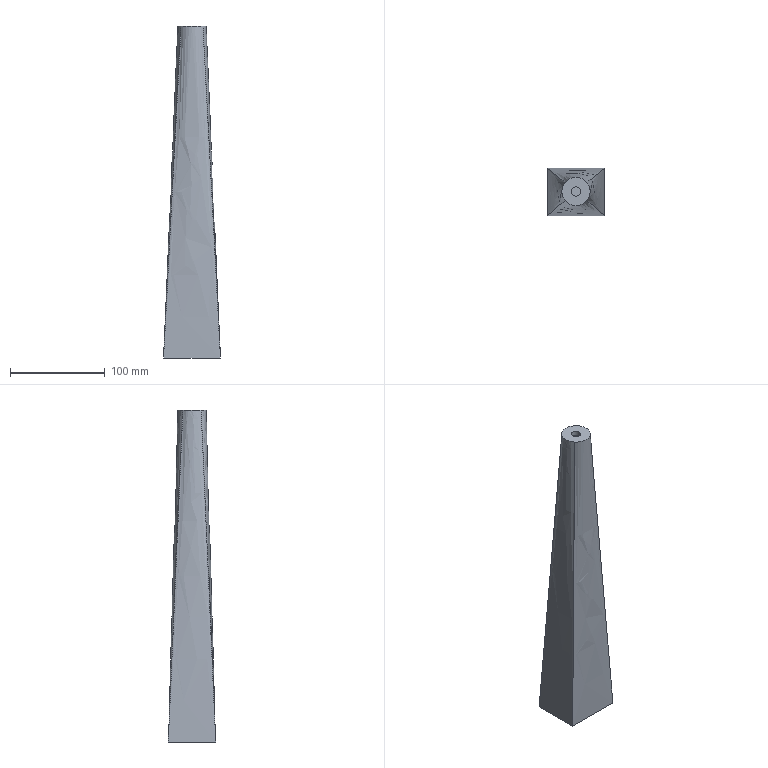Part | SolidWorks | features Blend 1, Cut 1 | 1 solid | 9 faces | box 60 x 50 x 350 mm | volume 603883 mm3 | spline 4 | plane 3 | cylinder 2 | commonest cylinder face diameters 9.779 x2
STEP:
#1=CARTESIAN_POINT('',(-4.89,0.,-5.));
#2=VERTEX_POINT('',#1);
#3=CARTESIAN_POINT('',(4.89,0.,-5.));
#4=VERTEX_POINT('',#3);
#5=CARTESIAN_POINT('',(0.,0.,-5.));
#6=DIRECTION('',(0.,0.,1.));
#7=DIRECTION('',(1.,0.,0.));
#8=AXIS2_PLACEMENT_3D('',#5,#6,#7);
#9=CIRCLE('',#8,4.89);
#10=EDGE_CURVE('',#2,#4,#9,.T.);
#11=ORIENTED_EDGE('',*,*,#10,.F.);
#12=CARTESIAN_POINT('',(-4.89,0.,0.));
#13=VERTEX_POINT('',#12);
#14=CARTESIAN_POINT('',(-4.89,0.,-5.));
#15=DIRECTION('',(0.,0.,1.));
#16=VECTOR('',#15,1000.);
#17=LINE('',#14,#16);
#18=EDGE_CURVE('',#2,#13,#17,.T.);
#19=ORIENTED_EDGE('',*,*,#18,.T.);
#20=CARTESIAN_POINT('',(4.89,0.,0.));
#21=VERTEX_POINT('',#20);
#22=CARTESIAN_POINT('',(0.,0.,0.));
#23=DIRECTION('',(0.,0.,1.));
#24=DIRECTION('',(1.,0.,0.));
#25=AXIS2_PLACEMENT_3D('',#22,#23,#24);
#26=CIRCLE('',#25,4.89);
#27=EDGE_CURVE('',#13,#21,#26,.T.);
#28=ORIENTED_EDGE('',*,*,#27,.T.);
#29=CARTESIAN_POINT('',(4.89,0.,-5.));
#30=DIRECTION('',(0.,0.,1.));
#31=VECTOR('',#30,1000.);
#32=LINE('',#29,#31);
#33=EDGE_CURVE('',#4,#21,#32,.T.);
#34=ORIENTED_EDGE('',*,*,#33,.F.);
#35=EDGE_LOOP('',(#11,#19,#28,#34));
#36=FACE_OUTER_BOUND('',#35,.T.);
#37=CARTESIAN_POINT('',(0.,0.,-5.));
#38=DIRECTION('',(0.,0.,1.));
#39=DIRECTION('',(1.,0.,0.));
#40=AXIS2_PLACEMENT_3D('',#37,#38,#39);
#41=CYLINDRICAL_SURFACE('',#40,4.89);
#42=ADVANCED_FACE('',(#36),#41,.F.);
#43=CARTESIAN_POINT('',(0.,0.,0.));
#44=DIRECTION('',(0.,0.,1.));
#45=DIRECTION('',(1.,0.,0.));
#46=AXIS2_PLACEMENT_3D('',#43,#44,#45);
#47=CIRCLE('',#46,4.89);
#48=EDGE_CURVE('',#21,#13,#47,.T.);
#49=ORIENTED_EDGE('',*,*,#48,.F.);
#50=ORIENTED_EDGE('',*,*,#27,.F.);
#51=EDGE_LOOP('',(#49,#50));
#52=FACE_BOUND('',#51,.T.);
#53=CARTESIAN_POINT('',(11.523,-9.603,0.));
#54=VERTEX_POINT('',#53);
#55=CARTESIAN_POINT('',(11.523,9.603,0.));
#56=VERTEX_POINT('',#55);
#57=CARTESIAN_POINT('',(0.,0.,0.));
#58=DIRECTION('',(0.,0.,1.));
#59=DIRECTION('',(1.,0.,0.));
#60=AXIS2_PLACEMENT_3D('',#57,#58,#59);
#61=CIRCLE('',#60,15.);
#62=EDGE_CURVE('',#54,#56,#61,.T.);
#63=ORIENTED_EDGE('',*,*,#62,.T.);
#64=CARTESIAN_POINT('',(-11.523,9.603,0.));
#65=VERTEX_POINT('',#64);
#66=CARTESIAN_POINT('',(0.,0.,0.));
#67=DIRECTION('',(0.,0.,1.));
#68=DIRECTION('',(1.,0.,0.));
#69=AXIS2_PLACEMENT_3D('',#66,#67,#68);
#70=CIRCLE('',#69,15.);
#71=EDGE_CURVE('',#56,#65,#70,.T.);
#72=ORIENTED_EDGE('',*,*,#71,.T.);
#73=CARTESIAN_POINT('',(-11.523,-9.603,0.));
#74=VERTEX_POINT('',#73);
#75=CARTESIAN_POINT('',(0.,0.,0.));
#76=DIRECTION('',(0.,0.,1.));
#77=DIRECTION('',(1.,0.,0.));
#78=AXIS2_PLACEMENT_3D('',#75,#76,#77);
#79=CIRCLE('',#78,15.);
#80=EDGE_CURVE('',#65,#74,#79,.T.);
#81=ORIENTED_EDGE('',*,*,#80,.T.);
#82=CARTESIAN_POINT('',(0.,0.,0.));
#83=DIRECTION('',(0.,0.,1.));
#84=DIRECTION('',(1.,0.,0.));
#85=AXIS2_PLACEMENT_3D('',#82,#83,#84);
#86=CIRCLE('',#85,15.);
#87=EDGE_CURVE('',#74,#54,#86,.T.);
#88=ORIENTED_EDGE('',*,*,#87,.T.);
#89=EDGE_LOOP('',(#63,#72,#81,#88));
#90=FACE_OUTER_BOUND('',#89,.T.);
#91=CARTESIAN_POINT('',(0.,0.,0.));
#92=DIRECTION('',(0.,0.,1.));
#93=DIRECTION('',(1.,0.,0.));
#94=AXIS2_PLACEMENT_3D('',#91,#92,#93);
#95=PLANE('',#94);
#96=ADVANCED_FACE('',(#52,#90),#95,.T.);
#97=CARTESIAN_POINT('',(30.,-25.,-350.));
#98=VERTEX_POINT('',#97);
#99=CARTESIAN_POINT('',(30.,25.,-350.));
#100=VERTEX_POINT('',#99);
#101=CARTESIAN_POINT('',(30.,25.,-350.));
#102=DIRECTION('',(0.,1.,0.));
#103=VECTOR('',#102,1000.);
#104=LINE('',#101,#103);
#105=EDGE_CURVE('',#98,#100,#104,.T.);
#106=ORIENTED_EDGE('',*,*,#105,.F.);
#107=CARTESIAN_POINT('',(-30.,-25.,-350.));
#108=VERTEX_POINT('',#107);
#109=CARTESIAN_POINT('',(-30.,-25.,-350.));
#110=DIRECTION('',(1.,0.,0.));
#111=VECTOR('',#110,1000.);
#112=LINE('',#109,#111);
#113=EDGE_CURVE('',#108,#98,#112,.T.);
#114=ORIENTED_EDGE('',*,*,#113,.F.);
#115=CARTESIAN_POINT('',(-30.,25.,-350.));
#116=VERTEX_POINT('',#115);
#117=CARTESIAN_POINT('',(-30.,25.,-350.));
#118=DIRECTION('',(0.,-1.,0.));
#119=VECTOR('',#118,1000.);
#120=LINE('',#117,#119);
#121=EDGE_CURVE('',#116,#108,#120,.T.);
#122=ORIENTED_EDGE('',*,*,#121,.F.);
#123=CARTESIAN_POINT('',(-30.,25.,-350.));
#124=DIRECTION('',(-1.,0.,0.));
#125=VECTOR('',#124,1000.);
#126=LINE('',#123,#125);
#127=EDGE_CURVE('',#100,#116,#126,.T.);
#128=ORIENTED_EDGE('',*,*,#127,.F.);
#129=EDGE_LOOP('',(#106,#114,#122,#128));
#130=FACE_OUTER_BOUND('',#129,.T.);
#131=CARTESIAN_POINT('',(0.,0.,-350.));
#132=DIRECTION('',(0.,0.,1.));
#133=DIRECTION('',(1.,0.,0.));
#134=AXIS2_PLACEMENT_3D('',#131,#132,#133);
#135=PLANE('',#134);
#136=ADVANCED_FACE('',(#130),#135,.F.);
#137=ORIENTED_EDGE('',*,*,#127,.T.);
#138=CARTESIAN_POINT('',(-20.762,17.301,-175.));
#139=DIRECTION('',(0.05267,-0.04389,0.9976));
#140=VECTOR('',#139,1000.);
#141=LINE('',#138,#140);
#142=EDGE_CURVE('',#116,#65,#141,.T.);
#143=ORIENTED_EDGE('',*,*,#142,.T.);
#144=ORIENTED_EDGE('',*,*,#71,.F.);
#145=CARTESIAN_POINT('',(20.762,17.301,-175.));
#146=DIRECTION('',(0.05267,0.04389,-0.9976));
#147=VECTOR('',#146,1000.);
#148=LINE('',#145,#147);
#149=EDGE_CURVE('',#56,#100,#148,.T.);
#150=ORIENTED_EDGE('',*,*,#149,.T.);
#151=EDGE_LOOP('',(#137,#143,#144,#150));
#152=FACE_OUTER_BOUND('',#151,.T.);
#153=CARTESIAN_POINT('',(30.,25.,-350.));
#154=CARTESIAN_POINT('',(11.523,9.603,0.));
#155=CARTESIAN_POINT('',(27.5,25.,-350.));
#156=CARTESIAN_POINT('',(10.909,10.34,0.));
#157=CARTESIAN_POINT('',(25.,25.,-350.));
#158=CARTESIAN_POINT('',(10.194,11.053,0.));
#159=CARTESIAN_POINT('',(20.,25.,-350.));
#160=CARTESIAN_POINT('',(8.568,12.357,0.));
#161=CARTESIAN_POINT('',(17.5,25.,-350.));
#162=CARTESIAN_POINT('',(7.655,12.947,0.));
#163=CARTESIAN_POINT('',(12.5,25.,-350.));
#164=CARTESIAN_POINT('',(5.666,13.933,0.));
#165=CARTESIAN_POINT('',(10.,25.,-350.));
#166=CARTESIAN_POINT('',(4.589,14.327,0.));
#167=CARTESIAN_POINT('',(5.,25.,-350.));
#168=CARTESIAN_POINT('',(2.341,14.861,0.));
#169=CARTESIAN_POINT('',(2.5,25.,-350.));
#170=CARTESIAN_POINT('',(1.171,15.,0.));
#171=CARTESIAN_POINT('',(-2.5,25.,-350.));
#172=CARTESIAN_POINT('',(-1.171,15.,0.));
#173=CARTESIAN_POINT('',(-5.,25.,-350.));
#174=CARTESIAN_POINT('',(-2.341,14.861,0.));
#175=CARTESIAN_POINT('',(-10.,25.,-350.));
#176=CARTESIAN_POINT('',(-4.589,14.327,0.));
#177=CARTESIAN_POINT('',(-12.5,25.,-350.));
#178=CARTESIAN_POINT('',(-5.666,13.933,0.));
#179=CARTESIAN_POINT('',(-17.5,25.,-350.));
#180=CARTESIAN_POINT('',(-7.655,12.947,0.));
#181=CARTESIAN_POINT('',(-20.,25.,-350.));
#182=CARTESIAN_POINT('',(-8.568,12.357,0.));
#183=CARTESIAN_POINT('',(-25.,25.,-350.));
#184=CARTESIAN_POINT('',(-10.194,11.053,0.));
#185=CARTESIAN_POINT('',(-27.5,25.,-350.));
#186=CARTESIAN_POINT('',(-10.909,10.34,0.));
#187=CARTESIAN_POINT('',(-30.,25.,-350.));
#188=CARTESIAN_POINT('',(-11.523,9.603,0.));
#189=B_SPLINE_SURFACE_WITH_KNOTS('',3,1,((#153,#154),(#155,#156),(#157,#158),(#159,#160),(#161,#162),(#163,#164),(#165,#166),(#167,#168),(#169,#170),(#171,#172),(#173,#174),(#175,#176),(#177,#178),(#179,#180),(#181,#182),(#183,#184),(#185,#186),(#187,#188)),.UNSPECIFIED.,.F.,.F.,.F.,(4,2,2,2,2,2,2,2,4),(2,2),(0.,0.125,0.25,0.375,0.5,0.625,0.75,0.875,1.),(0.,1.),.UNSPECIFIED.);
#190=ADVANCED_FACE('',(#152),#189,.T.);
#191=ORIENTED_EDGE('',*,*,#121,.T.);
#192=CARTESIAN_POINT('',(-20.762,-17.301,-175.));
#193=DIRECTION('',(0.05267,0.04389,0.9976));
#194=VECTOR('',#193,1000.);
#195=LINE('',#192,#194);
#196=EDGE_CURVE('',#108,#74,#195,.T.);
#197=ORIENTED_EDGE('',*,*,#196,.T.);
#198=ORIENTED_EDGE('',*,*,#80,.F.);
#199=ORIENTED_EDGE('',*,*,#142,.F.);
#200=EDGE_LOOP('',(#191,#197,#198,#199));
#201=FACE_OUTER_BOUND('',#200,.T.);
#202=CARTESIAN_POINT('',(-30.,25.,-350.));
#203=CARTESIAN_POINT('',(-11.523,9.603,0.));
#204=CARTESIAN_POINT('',(-30.,22.917,-350.));
#205=CARTESIAN_POINT('',(-12.036,8.988,0.));
#206=CARTESIAN_POINT('',(-30.,20.833,-350.));
#207=CARTESIAN_POINT('',(-12.514,8.314,0.));
#208=CARTESIAN_POINT('',(-30.,16.667,-350.));
#209=CARTESIAN_POINT('',(-13.366,6.86,0.));
#210=CARTESIAN_POINT('',(-30.,14.583,-350.));
#211=CARTESIAN_POINT('',(-13.741,6.079,0.));
#212=CARTESIAN_POINT('',(-30.,10.417,-350.));
#213=CARTESIAN_POINT('',(-14.355,4.438,0.));
#214=CARTESIAN_POINT('',(-30.,8.333,-350.));
#215=CARTESIAN_POINT('',(-14.595,3.576,0.));
#216=CARTESIAN_POINT('',(-30.,4.167,-350.));
#217=CARTESIAN_POINT('',(-14.917,1.81,0.));
#218=CARTESIAN_POINT('',(-30.,2.083,-350.));
#219=CARTESIAN_POINT('',(-15.,0.9051,0.));
#220=CARTESIAN_POINT('',(-30.,-2.083,-350.));
#221=CARTESIAN_POINT('',(-15.,-0.9051,0.));
#222=CARTESIAN_POINT('',(-30.,-4.167,-350.));
#223=CARTESIAN_POINT('',(-14.917,-1.81,0.));
#224=CARTESIAN_POINT('',(-30.,-8.333,-350.));
#225=CARTESIAN_POINT('',(-14.595,-3.576,0.));
#226=CARTESIAN_POINT('',(-30.,-10.417,-350.));
#227=CARTESIAN_POINT('',(-14.355,-4.438,0.));
#228=CARTESIAN_POINT('',(-30.,-14.583,-350.));
#229=CARTESIAN_POINT('',(-13.741,-6.079,0.));
#230=CARTESIAN_POINT('',(-30.,-16.667,-350.));
#231=CARTESIAN_POINT('',(-13.366,-6.86,0.));
#232=CARTESIAN_POINT('',(-30.,-20.833,-350.));
#233=CARTESIAN_POINT('',(-12.514,-8.314,0.));
#234=CARTESIAN_POINT('',(-30.,-22.917,-350.));
#235=CARTESIAN_POINT('',(-12.036,-8.988,0.));
#236=CARTESIAN_POINT('',(-30.,-25.,-350.));
#237=CARTESIAN_POINT('',(-11.523,-9.603,0.));
#238=B_SPLINE_SURFACE_WITH_KNOTS('',3,1,((#202,#203),(#204,#205),(#206,#207),(#208,#209),(#210,#211),(#212,#213),(#214,#215),(#216,#217),(#218,#219),(#220,#221),(#222,#223),(#224,#225),(#226,#227),(#228,#229),(#230,#231),(#232,#233),(#234,#235),(#236,#237)),.UNSPECIFIED.,.F.,.F.,.F.,(4,2,2,2,2,2,2,2,4),(2,2),(0.,0.125,0.25,0.375,0.5,0.625,0.75,0.875,1.),(0.,1.),.UNSPECIFIED.);
#239=ADVANCED_FACE('',(#201),#238,.T.);
#240=ORIENTED_EDGE('',*,*,#105,.T.);
#241=ORIENTED_EDGE('',*,*,#149,.F.);
#242=ORIENTED_EDGE('',*,*,#62,.F.);
#243=CARTESIAN_POINT('',(20.762,-17.301,-175.));
#244=DIRECTION('',(-0.05267,0.04389,0.9976));
#245=VECTOR('',#244,1000.);
#246=LINE('',#243,#245);
#247=EDGE_CURVE('',#98,#54,#246,.T.);
#248=ORIENTED_EDGE('',*,*,#247,.F.);
#249=EDGE_LOOP('',(#240,#241,#242,#248));
#250=FACE_OUTER_BOUND('',#249,.T.);
#251=CARTESIAN_POINT('',(30.,-25.,-350.));
#252=CARTESIAN_POINT('',(11.523,-9.603,0.));
#253=CARTESIAN_POINT('',(30.,-22.917,-350.));
#254=CARTESIAN_POINT('',(12.036,-8.988,0.));
#255=CARTESIAN_POINT('',(30.,-20.833,-350.));
#256=CARTESIAN_POINT('',(12.514,-8.314,0.));
#257=CARTESIAN_POINT('',(30.,-16.667,-350.));
#258=CARTESIAN_POINT('',(13.366,-6.86,0.));
#259=CARTESIAN_POINT('',(30.,-14.583,-350.));
#260=CARTESIAN_POINT('',(13.741,-6.079,0.));
#261=CARTESIAN_POINT('',(30.,-10.417,-350.));
#262=CARTESIAN_POINT('',(14.355,-4.438,0.));
#263=CARTESIAN_POINT('',(30.,-8.333,-350.));
#264=CARTESIAN_POINT('',(14.595,-3.576,0.));
#265=CARTESIAN_POINT('',(30.,-4.167,-350.));
#266=CARTESIAN_POINT('',(14.917,-1.81,0.));
#267=CARTESIAN_POINT('',(30.,-2.083,-350.));
#268=CARTESIAN_POINT('',(15.,-0.9051,0.));
#269=CARTESIAN_POINT('',(30.,2.083,-350.));
#270=CARTESIAN_POINT('',(15.,0.9051,0.));
#271=CARTESIAN_POINT('',(30.,4.167,-350.));
#272=CARTESIAN_POINT('',(14.917,1.81,0.));
#273=CARTESIAN_POINT('',(30.,8.333,-350.));
#274=CARTESIAN_POINT('',(14.595,3.576,0.));
#275=CARTESIAN_POINT('',(30.,10.417,-350.));
#276=CARTESIAN_POINT('',(14.355,4.438,0.));
#277=CARTESIAN_POINT('',(30.,14.583,-350.));
#278=CARTESIAN_POINT('',(13.741,6.079,0.));
#279=CARTESIAN_POINT('',(30.,16.667,-350.));
#280=CARTESIAN_POINT('',(13.366,6.86,0.));
#281=CARTESIAN_POINT('',(30.,20.833,-350.));
#282=CARTESIAN_POINT('',(12.514,8.314,0.));
#283=CARTESIAN_POINT('',(30.,22.917,-350.));
#284=CARTESIAN_POINT('',(12.036,8.988,0.));
#285=CARTESIAN_POINT('',(30.,25.,-350.));
#286=CARTESIAN_POINT('',(11.523,9.603,0.));
#287=B_SPLINE_SURFACE_WITH_KNOTS('',3,1,((#251,#252),(#253,#254),(#255,#256),(#257,#258),(#259,#260),(#261,#262),(#263,#264),(#265,#266),(#267,#268),(#269,#270),(#271,#272),(#273,#274),(#275,#276),(#277,#278),(#279,#280),(#281,#282),(#283,#284),(#285,#286)),.UNSPECIFIED.,.F.,.F.,.F.,(4,2,2,2,2,2,2,2,4),(2,2),(0.,0.125,0.25,0.375,0.5,0.625,0.75,0.875,1.),(0.,1.),.UNSPECIFIED.);
#288=ADVANCED_FACE('',(#250),#287,.T.);
#289=ORIENTED_EDGE('',*,*,#113,.T.);
#290=ORIENTED_EDGE('',*,*,#247,.T.);
#291=ORIENTED_EDGE('',*,*,#87,.F.);
#292=ORIENTED_EDGE('',*,*,#196,.F.);
#293=EDGE_LOOP('',(#289,#290,#291,#292));
#294=FACE_OUTER_BOUND('',#293,.T.);
#295=CARTESIAN_POINT('',(-30.,-25.,-350.));
#296=CARTESIAN_POINT('',(-11.523,-9.603,0.));
#297=CARTESIAN_POINT('',(-27.5,-25.,-350.));
#298=CARTESIAN_POINT('',(-10.909,-10.34,0.));
#299=CARTESIAN_POINT('',(-25.,-25.,-350.));
#300=CARTESIAN_POINT('',(-10.194,-11.053,0.));
#301=CARTESIAN_POINT('',(-20.,-25.,-350.));
#302=CARTESIAN_POINT('',(-8.568,-12.357,0.));
#303=CARTESIAN_POINT('',(-17.5,-25.,-350.));
#304=CARTESIAN_POINT('',(-7.655,-12.947,0.));
#305=CARTESIAN_POINT('',(-12.5,-25.,-350.));
#306=CARTESIAN_POINT('',(-5.666,-13.933,0.));
#307=CARTESIAN_POINT('',(-10.,-25.,-350.));
#308=CARTESIAN_POINT('',(-4.589,-14.327,0.));
#309=CARTESIAN_POINT('',(-5.,-25.,-350.));
#310=CARTESIAN_POINT('',(-2.341,-14.861,0.));
#311=CARTESIAN_POINT('',(-2.5,-25.,-350.));
#312=CARTESIAN_POINT('',(-1.171,-15.,0.));
#313=CARTESIAN_POINT('',(2.5,-25.,-350.));
#314=CARTESIAN_POINT('',(1.171,-15.,0.));
#315=CARTESIAN_POINT('',(5.,-25.,-350.));
#316=CARTESIAN_POINT('',(2.341,-14.861,0.));
#317=CARTESIAN_POINT('',(10.,-25.,-350.));
#318=CARTESIAN_POINT('',(4.589,-14.327,0.));
#319=CARTESIAN_POINT('',(12.5,-25.,-350.));
#320=CARTESIAN_POINT('',(5.666,-13.933,0.));
#321=CARTESIAN_POINT('',(17.5,-25.,-350.));
#322=CARTESIAN_POINT('',(7.655,-12.947,0.));
#323=CARTESIAN_POINT('',(20.,-25.,-350.));
#324=CARTESIAN_POINT('',(8.568,-12.357,0.));
#325=CARTESIAN_POINT('',(25.,-25.,-350.));
#326=CARTESIAN_POINT('',(10.194,-11.053,0.));
#327=CARTESIAN_POINT('',(27.5,-25.,-350.));
#328=CARTESIAN_POINT('',(10.909,-10.34,0.));
#329=CARTESIAN_POINT('',(30.,-25.,-350.));
#330=CARTESIAN_POINT('',(11.523,-9.603,0.));
#331=B_SPLINE_SURFACE_WITH_KNOTS('',3,1,((#295,#296),(#297,#298),(#299,#300),(#301,#302),(#303,#304),(#305,#306),(#307,#308),(#309,#310),(#311,#312),(#313,#314),(#315,#316),(#317,#318),(#319,#320),(#321,#322),(#323,#324),(#325,#326),(#327,#328),(#329,#330)),.UNSPECIFIED.,.F.,.F.,.F.,(4,2,2,2,2,2,2,2,4),(2,2),(0.,0.125,0.25,0.375,0.5,0.625,0.75,0.875,1.),(0.,1.),.UNSPECIFIED.);
#332=ADVANCED_FACE('',(#294),#331,.T.);
#333=ORIENTED_EDGE('',*,*,#18,.F.);
#334=CARTESIAN_POINT('',(0.,0.,-5.));
#335=DIRECTION('',(0.,0.,1.));
#336=DIRECTION('',(1.,0.,0.));
#337=AXIS2_PLACEMENT_3D('',#334,#335,#336);
#338=CIRCLE('',#337,4.89);
#339=EDGE_CURVE('',#4,#2,#338,.T.);
#340=ORIENTED_EDGE('',*,*,#339,.F.);
#341=ORIENTED_EDGE('',*,*,#33,.T.);
#342=ORIENTED_EDGE('',*,*,#48,.T.);
#343=EDGE_LOOP('',(#333,#340,#341,#342));
#344=FACE_OUTER_BOUND('',#343,.T.);
#345=CARTESIAN_POINT('',(0.,0.,-5.));
#346=DIRECTION('',(0.,0.,1.));
#347=DIRECTION('',(1.,0.,0.));
#348=AXIS2_PLACEMENT_3D('',#345,#346,#347);
#349=CYLINDRICAL_SURFACE('',#348,4.89);
#350=ADVANCED_FACE('',(#344),#349,.F.);
#351=ORIENTED_EDGE('',*,*,#339,.T.);
#352=ORIENTED_EDGE('',*,*,#10,.T.);
#353=EDGE_LOOP('',(#351,#352));
#354=FACE_OUTER_BOUND('',#353,.T.);
#355=CARTESIAN_POINT('',(0.,0.,-5.));
#356=DIRECTION('',(0.,0.,1.));
#357=DIRECTION('',(1.,0.,0.));
#358=AXIS2_PLACEMENT_3D('',#355,#356,#357);
#359=PLANE('',#358);
#360=ADVANCED_FACE('',(#354),#359,.T.);
#361=CLOSED_SHELL('',(#42,#96,#136,#190,#239,#288,#332,#350,#360));
#362=MANIFOLD_SOLID_BREP('',#361);
#363=CARTESIAN_POINT('',(0.,0.,0.));
#364=DIRECTION('',(0.,0.,1.));
#365=DIRECTION('',(1.,0.,0.));
#366=AXIS2_PLACEMENT_3D('',#363,#364,#365);
#367=(LENGTH_UNIT()NAMED_UNIT(*)SI_UNIT(.MILLI.,.METRE.));
#368=UNCERTAINTY_MEASURE_WITH_UNIT(LENGTH_MEASURE(0.00001),#367,'','');
#369=(NAMED_UNIT(*)PLANE_ANGLE_UNIT()SI_UNIT($,.RADIAN.));
#370=(NAMED_UNIT(*)SI_UNIT($,.STERADIAN.)SOLID_ANGLE_UNIT());
#371=(GEOMETRIC_REPRESENTATION_CONTEXT(3)GLOBAL_UNCERTAINTY_ASSIGNED_CONTEXT((#368))GLOBAL_UNIT_ASSIGNED_CONTEXT((#367,#369,#370))REPRESENTATION_CONTEXT('',''));
#372=ADVANCED_BREP_SHAPE_REPRESENTATION('',(#362,#366),#371);